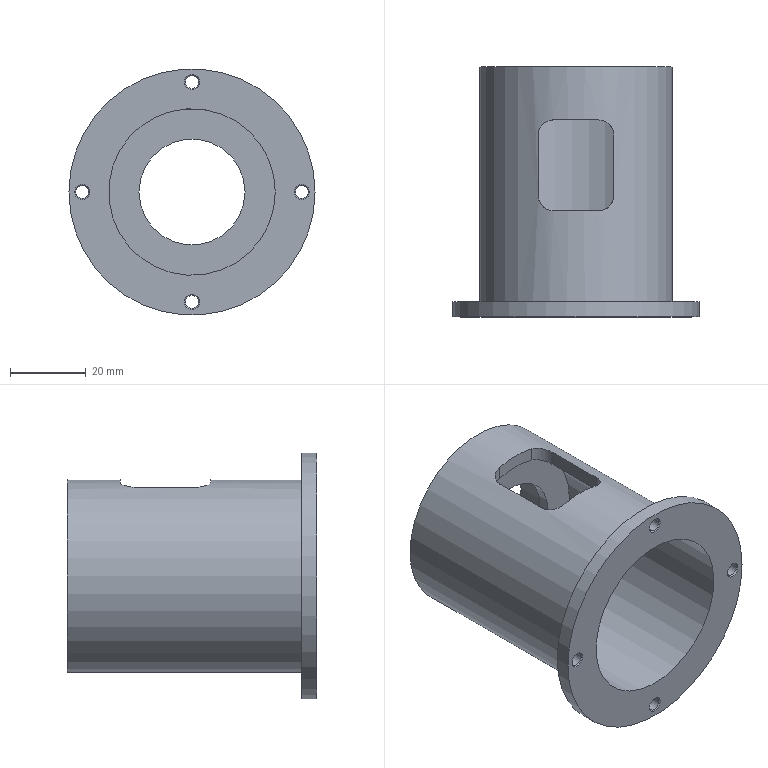Part | NX | features DATUM_CSYS 7, SKETCH 6, EXTRUDE 5, SIMPLE HOLE 4, BLEND 1, HOLE PACKAGE 1 | 1 solid | 30 faces | box 65 x 66 x 65 mm | volume 46902 mm3 | cylinder 13 | plane 9 | cone 8 | commonest cylinder face diameters 3.4 x4 8 x4 28 x1 32 x1 44 x1 51 x1
STEP:
#1=CARTESIAN_POINT('',(22.,54.,0.));
#2=VERTEX_POINT('',#1);
#3=CARTESIAN_POINT('',(0.,54.,0.));
#4=DIRECTION('',(0.,1.,0.));
#5=DIRECTION('',(1.,0.,0.));
#6=AXIS2_PLACEMENT_3D('',#3,#4,#5);
#7=CIRCLE('',#6,22.);
#8=EDGE_CURVE('',#2,#2,#7,.T.);
#9=ORIENTED_EDGE('',*,*,#8,.T.);
#10=EDGE_LOOP('',(#9));
#11=FACE_BOUND('',#10,.T.);
#12=CARTESIAN_POINT('',(22.,0.,0.));
#13=VERTEX_POINT('',#12);
#14=CARTESIAN_POINT('',(0.,0.,0.));
#15=DIRECTION('',(0.,-1.,0.));
#16=DIRECTION('',(1.,0.,0.));
#17=AXIS2_PLACEMENT_3D('',#14,#15,#16);
#18=CIRCLE('',#17,22.);
#19=EDGE_CURVE('',#13,#13,#18,.T.);
#20=ORIENTED_EDGE('',*,*,#19,.T.);
#21=EDGE_LOOP('',(#20));
#22=FACE_BOUND('',#21,.T.);
#23=CARTESIAN_POINT('',(-10.,32.,19.596));
#24=VERTEX_POINT('',#23);
#25=CARTESIAN_POINT('',(-10.,48.,19.596));
#26=VERTEX_POINT('',#25);
#27=CARTESIAN_POINT('',(-10.,4.,19.596));
#28=DIRECTION('',(0.,-1.,0.));
#29=VECTOR('',#28,1000.);
#30=LINE('',#27,#29);
#31=EDGE_CURVE('',#24,#26,#30,.F.);
#32=ORIENTED_EDGE('',*,*,#31,.F.);
#33=CARTESIAN_POINT('',(-6.,28.,21.166));
#34=VERTEX_POINT('',#33);
#35=CARTESIAN_POINT('',(-10.,32.,19.596));
#36=CARTESIAN_POINT('',(-10.,30.905,19.596));
#37=CARTESIAN_POINT('',(-9.065,28.825,20.099));
#38=CARTESIAN_POINT('',(-7.052,28.,20.868));
#39=CARTESIAN_POINT('',(-6.,28.,21.166));
#40=B_SPLINE_CURVE_WITH_KNOTS('',3,(#35,#36,#37,#38,#39),.UNSPECIFIED.,.F.,.F.,(4,1,4),(0.,0.003234,0.006469),.UNSPECIFIED.);
#41=EDGE_CURVE('',#24,#34,#40,.T.);
#42=ORIENTED_EDGE('',*,*,#41,.T.);
#43=CARTESIAN_POINT('',(6.,28.,21.166));
#44=VERTEX_POINT('',#43);
#45=CARTESIAN_POINT('',(0.,28.,0.));
#46=DIRECTION('',(0.,1.,0.));
#47=DIRECTION('',(0.,0.,1.));
#48=AXIS2_PLACEMENT_3D('',#45,#46,#47);
#49=CIRCLE('',#48,22.);
#50=EDGE_CURVE('',#44,#34,#49,.F.);
#51=ORIENTED_EDGE('',*,*,#50,.F.);
#52=CARTESIAN_POINT('',(10.,32.,19.596));
#53=VERTEX_POINT('',#52);
#54=CARTESIAN_POINT('',(6.,28.,21.166));
#55=CARTESIAN_POINT('',(7.053,28.,20.868));
#56=CARTESIAN_POINT('',(9.063,28.824,20.1));
#57=CARTESIAN_POINT('',(10.,30.904,19.596));
#58=CARTESIAN_POINT('',(10.,32.,19.596));
#59=B_SPLINE_CURVE_WITH_KNOTS('',3,(#54,#55,#56,#57,#58),.UNSPECIFIED.,.F.,.F.,(4,1,4),(0.,0.003235,0.006469),.UNSPECIFIED.);
#60=EDGE_CURVE('',#44,#53,#59,.T.);
#61=ORIENTED_EDGE('',*,*,#60,.T.);
#62=CARTESIAN_POINT('',(10.,48.,19.596));
#63=VERTEX_POINT('',#62);
#64=CARTESIAN_POINT('',(10.,4.,19.596));
#65=DIRECTION('',(0.,-1.,0.));
#66=VECTOR('',#65,1000.);
#67=LINE('',#64,#66);
#68=EDGE_CURVE('',#63,#53,#67,.T.);
#69=ORIENTED_EDGE('',*,*,#68,.F.);
#70=CARTESIAN_POINT('',(6.,52.,21.166));
#71=VERTEX_POINT('',#70);
#72=CARTESIAN_POINT('',(10.,48.,19.596));
#73=CARTESIAN_POINT('',(10.,49.095,19.596));
#74=CARTESIAN_POINT('',(9.065,51.175,20.099));
#75=CARTESIAN_POINT('',(7.052,52.,20.868));
#76=CARTESIAN_POINT('',(6.,52.,21.166));
#77=B_SPLINE_CURVE_WITH_KNOTS('',3,(#72,#73,#74,#75,#76),.UNSPECIFIED.,.F.,.F.,(4,1,4),(0.,0.003234,0.006469),.UNSPECIFIED.);
#78=EDGE_CURVE('',#63,#71,#77,.T.);
#79=ORIENTED_EDGE('',*,*,#78,.T.);
#80=CARTESIAN_POINT('',(-6.,52.,21.166));
#81=VERTEX_POINT('',#80);
#82=CARTESIAN_POINT('',(0.,52.,0.));
#83=DIRECTION('',(0.,-1.,0.));
#84=DIRECTION('',(0.,0.,-1.));
#85=AXIS2_PLACEMENT_3D('',#82,#83,#84);
#86=CIRCLE('',#85,22.);
#87=EDGE_CURVE('',#81,#71,#86,.F.);
#88=ORIENTED_EDGE('',*,*,#87,.F.);
#89=CARTESIAN_POINT('',(-6.,52.,21.166));
#90=CARTESIAN_POINT('',(-7.053,52.,20.868));
#91=CARTESIAN_POINT('',(-9.063,51.176,20.1));
#92=CARTESIAN_POINT('',(-10.,49.096,19.596));
#93=CARTESIAN_POINT('',(-10.,48.,19.596));
#94=B_SPLINE_CURVE_WITH_KNOTS('',3,(#89,#90,#91,#92,#93),.UNSPECIFIED.,.F.,.F.,(4,1,4),(0.,0.003235,0.006469),.UNSPECIFIED.);
#95=EDGE_CURVE('',#81,#26,#94,.T.);
#96=ORIENTED_EDGE('',*,*,#95,.T.);
#97=EDGE_LOOP('',(#32,#42,#51,#61,#69,#79,#88,#96));
#98=FACE_BOUND('',#97,.T.);
#99=CARTESIAN_POINT('',(0.,4.,0.));
#100=DIRECTION('',(0.,-1.,0.));
#101=DIRECTION('',(0.,0.,-1.));
#102=AXIS2_PLACEMENT_3D('',#99,#100,#101);
#103=CYLINDRICAL_SURFACE('',#102,22.);
#104=ADVANCED_FACE('',(#11,#22,#98),#103,.F.);
#105=CARTESIAN_POINT('',(25.5,66.,0.));
#106=VERTEX_POINT('',#105);
#107=CARTESIAN_POINT('',(0.,66.,0.));
#108=DIRECTION('',(0.,1.,0.));
#109=DIRECTION('',(1.,0.,0.));
#110=AXIS2_PLACEMENT_3D('',#107,#108,#109);
#111=CIRCLE('',#110,25.5);
#112=EDGE_CURVE('',#106,#106,#111,.T.);
#113=ORIENTED_EDGE('',*,*,#112,.F.);
#114=EDGE_LOOP('',(#113));
#115=FACE_BOUND('',#114,.T.);
#116=CARTESIAN_POINT('',(25.5,4.,0.));
#117=VERTEX_POINT('',#116);
#118=CARTESIAN_POINT('',(0.,4.,0.));
#119=DIRECTION('',(0.,1.,0.));
#120=DIRECTION('',(1.,0.,0.));
#121=AXIS2_PLACEMENT_3D('',#118,#119,#120);
#122=CIRCLE('',#121,25.5);
#123=EDGE_CURVE('',#117,#117,#122,.T.);
#124=ORIENTED_EDGE('',*,*,#123,.T.);
#125=EDGE_LOOP('',(#124));
#126=FACE_BOUND('',#125,.T.);
#127=CARTESIAN_POINT('',(-10.,48.,23.457));
#128=VERTEX_POINT('',#127);
#129=CARTESIAN_POINT('',(-10.,32.,23.457));
#130=VERTEX_POINT('',#129);
#131=CARTESIAN_POINT('',(-10.,54.,23.457));
#132=DIRECTION('',(0.,-1.,0.));
#133=VECTOR('',#132,1000.);
#134=LINE('',#131,#133);
#135=EDGE_CURVE('',#128,#130,#134,.T.);
#136=ORIENTED_EDGE('',*,*,#135,.F.);
#137=CARTESIAN_POINT('',(-6.,52.,24.784));
#138=VERTEX_POINT('',#137);
#139=CARTESIAN_POINT('',(-10.,48.,23.457));
#140=CARTESIAN_POINT('',(-10.,49.084,23.457));
#141=CARTESIAN_POINT('',(-9.082,51.163,23.871));
#142=CARTESIAN_POINT('',(-7.052,52.,24.529));
#143=CARTESIAN_POINT('',(-6.,52.,24.784));
#144=B_SPLINE_CURVE_WITH_KNOTS('',3,(#139,#140,#141,#142,#143),.UNSPECIFIED.,.F.,.F.,(4,1,4),(0.,0.003204,0.006407),.UNSPECIFIED.);
#145=EDGE_CURVE('',#128,#138,#144,.T.);
#146=ORIENTED_EDGE('',*,*,#145,.T.);
#147=CARTESIAN_POINT('',(6.,52.,24.784));
#148=VERTEX_POINT('',#147);
#149=CARTESIAN_POINT('',(0.,52.,0.));
#150=DIRECTION('',(0.,-1.,0.));
#151=DIRECTION('',(0.,0.,-1.));
#152=AXIS2_PLACEMENT_3D('',#149,#150,#151);
#153=CIRCLE('',#152,25.5);
#154=EDGE_CURVE('',#148,#138,#153,.T.);
#155=ORIENTED_EDGE('',*,*,#154,.F.);
#156=CARTESIAN_POINT('',(10.,48.,23.457));
#157=VERTEX_POINT('',#156);
#158=CARTESIAN_POINT('',(6.,52.,24.784));
#159=CARTESIAN_POINT('',(7.053,52.,24.529));
#160=CARTESIAN_POINT('',(9.079,51.165,23.871));
#161=CARTESIAN_POINT('',(10.,49.085,23.457));
#162=CARTESIAN_POINT('',(10.,48.,23.457));
#163=B_SPLINE_CURVE_WITH_KNOTS('',3,(#158,#159,#160,#161,#162),.UNSPECIFIED.,.F.,.F.,(4,1,4),(0.,0.003204,0.006407),.UNSPECIFIED.);
#164=EDGE_CURVE('',#148,#157,#163,.T.);
#165=ORIENTED_EDGE('',*,*,#164,.T.);
#166=CARTESIAN_POINT('',(10.,32.,23.457));
#167=VERTEX_POINT('',#166);
#168=CARTESIAN_POINT('',(10.,54.,23.457));
#169=DIRECTION('',(0.,-1.,0.));
#170=VECTOR('',#169,1000.);
#171=LINE('',#168,#170);
#172=EDGE_CURVE('',#167,#157,#171,.F.);
#173=ORIENTED_EDGE('',*,*,#172,.F.);
#174=CARTESIAN_POINT('',(6.,28.,24.784));
#175=VERTEX_POINT('',#174);
#176=CARTESIAN_POINT('',(10.,32.,23.457));
#177=CARTESIAN_POINT('',(10.,30.916,23.457));
#178=CARTESIAN_POINT('',(9.082,28.837,23.871));
#179=CARTESIAN_POINT('',(7.052,28.,24.529));
#180=CARTESIAN_POINT('',(6.,28.,24.784));
#181=B_SPLINE_CURVE_WITH_KNOTS('',3,(#176,#177,#178,#179,#180),.UNSPECIFIED.,.F.,.F.,(4,1,4),(0.,0.003204,0.006407),.UNSPECIFIED.);
#182=EDGE_CURVE('',#167,#175,#181,.T.);
#183=ORIENTED_EDGE('',*,*,#182,.T.);
#184=CARTESIAN_POINT('',(-6.,28.,24.784));
#185=VERTEX_POINT('',#184);
#186=CARTESIAN_POINT('',(0.,28.,0.));
#187=DIRECTION('',(0.,1.,0.));
#188=DIRECTION('',(0.,0.,1.));
#189=AXIS2_PLACEMENT_3D('',#186,#187,#188);
#190=CIRCLE('',#189,25.5);
#191=EDGE_CURVE('',#185,#175,#190,.T.);
#192=ORIENTED_EDGE('',*,*,#191,.F.);
#193=CARTESIAN_POINT('',(-6.,28.,24.784));
#194=CARTESIAN_POINT('',(-7.053,28.,24.529));
#195=CARTESIAN_POINT('',(-9.079,28.835,23.871));
#196=CARTESIAN_POINT('',(-10.,30.915,23.457));
#197=CARTESIAN_POINT('',(-10.,32.,23.457));
#198=B_SPLINE_CURVE_WITH_KNOTS('',3,(#193,#194,#195,#196,#197),.UNSPECIFIED.,.F.,.F.,(4,1,4),(0.,0.003204,0.006407),.UNSPECIFIED.);
#199=EDGE_CURVE('',#185,#130,#198,.T.);
#200=ORIENTED_EDGE('',*,*,#199,.T.);
#201=EDGE_LOOP('',(#136,#146,#155,#165,#173,#183,#192,#200));
#202=FACE_BOUND('',#201,.T.);
#203=CARTESIAN_POINT('',(0.,54.,0.));
#204=DIRECTION('',(0.,-1.,0.));
#205=DIRECTION('',(0.,0.,-1.));
#206=AXIS2_PLACEMENT_3D('',#203,#204,#205);
#207=CYLINDRICAL_SURFACE('',#206,25.5);
#208=ADVANCED_FACE('',(#115,#126,#202),#207,.T.);
#209=CARTESIAN_POINT('',(14.,57.,0.));
#210=VERTEX_POINT('',#209);
#211=CARTESIAN_POINT('',(0.,57.,0.));
#212=DIRECTION('',(0.,1.,0.));
#213=DIRECTION('',(1.,0.,0.));
#214=AXIS2_PLACEMENT_3D('',#211,#212,#213);
#215=CIRCLE('',#214,14.);
#216=EDGE_CURVE('',#210,#210,#215,.T.);
#217=ORIENTED_EDGE('',*,*,#216,.F.);
#218=EDGE_LOOP('',(#217));
#219=FACE_BOUND('',#218,.T.);
#220=CARTESIAN_POINT('',(16.,57.,0.));
#221=VERTEX_POINT('',#220);
#222=CARTESIAN_POINT('',(0.,57.,0.));
#223=DIRECTION('',(0.,1.,0.));
#224=DIRECTION('',(1.,0.,0.));
#225=AXIS2_PLACEMENT_3D('',#222,#223,#224);
#226=CIRCLE('',#225,16.);
#227=EDGE_CURVE('',#221,#221,#226,.T.);
#228=ORIENTED_EDGE('',*,*,#227,.T.);
#229=EDGE_LOOP('',(#228));
#230=FACE_BOUND('',#229,.T.);
#231=CARTESIAN_POINT('',(0.,57.,0.));
#232=DIRECTION('',(0.,1.,0.));
#233=DIRECTION('',(0.,0.,1.));
#234=AXIS2_PLACEMENT_3D('',#231,#232,#233);
#235=PLANE('',#234);
#236=ADVANCED_FACE('',(#219,#230),#235,.T.);
#237=CARTESIAN_POINT('',(29.,4.,-2.));
#238=VERTEX_POINT('',#237);
#239=CARTESIAN_POINT('',(29.,4.,0.));
#240=DIRECTION('',(0.,-1.,0.));
#241=DIRECTION('',(0.,0.,-1.));
#242=AXIS2_PLACEMENT_3D('',#239,#240,#241);
#243=CIRCLE('',#242,2.);
#244=EDGE_CURVE('',#238,#238,#243,.T.);
#245=ORIENTED_EDGE('',*,*,#244,.T.);
#246=EDGE_LOOP('',(#245));
#247=FACE_BOUND('',#246,.T.);
#248=CARTESIAN_POINT('',(0.,4.,27.));
#249=VERTEX_POINT('',#248);
#250=CARTESIAN_POINT('',(0.,4.,29.));
#251=DIRECTION('',(0.,-1.,0.));
#252=DIRECTION('',(0.,0.,-1.));
#253=AXIS2_PLACEMENT_3D('',#250,#251,#252);
#254=CIRCLE('',#253,2.);
#255=EDGE_CURVE('',#249,#249,#254,.T.);
#256=ORIENTED_EDGE('',*,*,#255,.T.);
#257=EDGE_LOOP('',(#256));
#258=FACE_BOUND('',#257,.T.);
#259=CARTESIAN_POINT('',(0.,4.,-31.));
#260=VERTEX_POINT('',#259);
#261=CARTESIAN_POINT('',(0.,4.,-29.));
#262=DIRECTION('',(0.,-1.,0.));
#263=DIRECTION('',(0.,0.,-1.));
#264=AXIS2_PLACEMENT_3D('',#261,#262,#263);
#265=CIRCLE('',#264,2.);
#266=EDGE_CURVE('',#260,#260,#265,.T.);
#267=ORIENTED_EDGE('',*,*,#266,.T.);
#268=EDGE_LOOP('',(#267));
#269=FACE_BOUND('',#268,.T.);
#270=CARTESIAN_POINT('',(-29.,4.,-2.));
#271=VERTEX_POINT('',#270);
#272=CARTESIAN_POINT('',(-29.,4.,0.));
#273=DIRECTION('',(0.,-1.,0.));
#274=DIRECTION('',(0.,0.,-1.));
#275=AXIS2_PLACEMENT_3D('',#272,#273,#274);
#276=CIRCLE('',#275,2.);
#277=EDGE_CURVE('',#271,#271,#276,.T.);
#278=ORIENTED_EDGE('',*,*,#277,.T.);
#279=EDGE_LOOP('',(#278));
#280=FACE_BOUND('',#279,.T.);
#281=CARTESIAN_POINT('',(32.5,4.,0.));
#282=VERTEX_POINT('',#281);
#283=CARTESIAN_POINT('',(0.,4.,0.));
#284=DIRECTION('',(0.,-1.,0.));
#285=DIRECTION('',(1.,0.,0.));
#286=AXIS2_PLACEMENT_3D('',#283,#284,#285);
#287=CIRCLE('',#286,32.5);
#288=EDGE_CURVE('',#282,#282,#287,.T.);
#289=ORIENTED_EDGE('',*,*,#288,.F.);
#290=EDGE_LOOP('',(#289));
#291=FACE_BOUND('',#290,.T.);
#292=ORIENTED_EDGE('',*,*,#123,.F.);
#293=EDGE_LOOP('',(#292));
#294=FACE_BOUND('',#293,.T.);
#295=CARTESIAN_POINT('',(0.,4.,0.));
#296=DIRECTION('',(0.,-1.,0.));
#297=DIRECTION('',(0.,0.,-1.));
#298=AXIS2_PLACEMENT_3D('',#295,#296,#297);
#299=PLANE('',#298);
#300=ADVANCED_FACE('',(#247,#258,#269,#280,#291,#294),#299,.F.);
#301=ORIENTED_EDGE('',*,*,#288,.T.);
#302=EDGE_LOOP('',(#301));
#303=FACE_BOUND('',#302,.T.);
#304=CARTESIAN_POINT('',(32.5,0.,0.));
#305=VERTEX_POINT('',#304);
#306=CARTESIAN_POINT('',(0.,0.,0.));
#307=DIRECTION('',(0.,-1.,0.));
#308=DIRECTION('',(1.,0.,0.));
#309=AXIS2_PLACEMENT_3D('',#306,#307,#308);
#310=CIRCLE('',#309,32.5);
#311=EDGE_CURVE('',#305,#305,#310,.T.);
#312=ORIENTED_EDGE('',*,*,#311,.F.);
#313=EDGE_LOOP('',(#312));
#314=FACE_BOUND('',#313,.T.);
#315=CARTESIAN_POINT('',(0.,4.,0.));
#316=DIRECTION('',(0.,-1.,0.));
#317=DIRECTION('',(0.,0.,-1.));
#318=AXIS2_PLACEMENT_3D('',#315,#316,#317);
#319=CYLINDRICAL_SURFACE('',#318,32.5);
#320=ADVANCED_FACE('',(#303,#314),#319,.T.);
#321=CARTESIAN_POINT('',(29.,0.,-2.));
#322=VERTEX_POINT('',#321);
#323=CARTESIAN_POINT('',(29.,0.,0.));
#324=DIRECTION('',(0.,-1.,0.));
#325=DIRECTION('',(0.,0.,-1.));
#326=AXIS2_PLACEMENT_3D('',#323,#324,#325);
#327=CIRCLE('',#326,2.);
#328=EDGE_CURVE('',#322,#322,#327,.F.);
#329=ORIENTED_EDGE('',*,*,#328,.T.);
#330=EDGE_LOOP('',(#329));
#331=FACE_BOUND('',#330,.T.);
#332=CARTESIAN_POINT('',(0.,0.,27.));
#333=VERTEX_POINT('',#332);
#334=CARTESIAN_POINT('',(0.,0.,29.));
#335=DIRECTION('',(0.,-1.,0.));
#336=DIRECTION('',(0.,0.,-1.));
#337=AXIS2_PLACEMENT_3D('',#334,#335,#336);
#338=CIRCLE('',#337,2.);
#339=EDGE_CURVE('',#333,#333,#338,.F.);
#340=ORIENTED_EDGE('',*,*,#339,.T.);
#341=EDGE_LOOP('',(#340));
#342=FACE_BOUND('',#341,.T.);
#343=CARTESIAN_POINT('',(0.,0.,-31.));
#344=VERTEX_POINT('',#343);
#345=CARTESIAN_POINT('',(0.,0.,-29.));
#346=DIRECTION('',(0.,-1.,0.));
#347=DIRECTION('',(0.,0.,-1.));
#348=AXIS2_PLACEMENT_3D('',#345,#346,#347);
#349=CIRCLE('',#348,2.);
#350=EDGE_CURVE('',#344,#344,#349,.F.);
#351=ORIENTED_EDGE('',*,*,#350,.T.);
#352=EDGE_LOOP('',(#351));
#353=FACE_BOUND('',#352,.T.);
#354=CARTESIAN_POINT('',(-29.,0.,-2.));
#355=VERTEX_POINT('',#354);
#356=CARTESIAN_POINT('',(-29.,0.,0.));
#357=DIRECTION('',(0.,-1.,0.));
#358=DIRECTION('',(0.,0.,-1.));
#359=AXIS2_PLACEMENT_3D('',#356,#357,#358);
#360=CIRCLE('',#359,2.);
#361=EDGE_CURVE('',#355,#355,#360,.F.);
#362=ORIENTED_EDGE('',*,*,#361,.T.);
#363=EDGE_LOOP('',(#362));
#364=FACE_BOUND('',#363,.T.);
#365=ORIENTED_EDGE('',*,*,#311,.T.);
#366=EDGE_LOOP('',(#365));
#367=FACE_BOUND('',#366,.T.);
#368=ORIENTED_EDGE('',*,*,#19,.F.);
#369=EDGE_LOOP('',(#368));
#370=FACE_BOUND('',#369,.T.);
#371=CARTESIAN_POINT('',(0.,0.,0.));
#372=DIRECTION('',(0.,-1.,0.));
#373=DIRECTION('',(0.,0.,-1.));
#374=AXIS2_PLACEMENT_3D('',#371,#372,#373);
#375=PLANE('',#374);
#376=ADVANCED_FACE('',(#331,#342,#353,#364,#367,#370),#375,.T.);
#377=ORIENTED_EDGE('',*,*,#216,.T.);
#378=EDGE_LOOP('',(#377));
#379=FACE_BOUND('',#378,.T.);
#380=CARTESIAN_POINT('',(14.,54.,0.));
#381=VERTEX_POINT('',#380);
#382=CARTESIAN_POINT('',(0.,54.,0.));
#383=DIRECTION('',(0.,1.,0.));
#384=DIRECTION('',(1.,0.,0.));
#385=AXIS2_PLACEMENT_3D('',#382,#383,#384);
#386=CIRCLE('',#385,14.);
#387=EDGE_CURVE('',#381,#381,#386,.T.);
#388=ORIENTED_EDGE('',*,*,#387,.F.);
#389=EDGE_LOOP('',(#388));
#390=FACE_BOUND('',#389,.T.);
#391=CARTESIAN_POINT('',(0.,57.,0.));
#392=DIRECTION('',(0.,-1.,0.));
#393=DIRECTION('',(0.,0.,-1.));
#394=AXIS2_PLACEMENT_3D('',#391,#392,#393);
#395=CYLINDRICAL_SURFACE('',#394,14.);
#396=ADVANCED_FACE('',(#379,#390),#395,.F.);
#397=ORIENTED_EDGE('',*,*,#8,.F.);
#398=EDGE_LOOP('',(#397));
#399=FACE_BOUND('',#398,.T.);
#400=ORIENTED_EDGE('',*,*,#387,.T.);
#401=EDGE_LOOP('',(#400));
#402=FACE_BOUND('',#401,.T.);
#403=CARTESIAN_POINT('',(0.,54.,0.));
#404=DIRECTION('',(0.,1.,0.));
#405=DIRECTION('',(0.,0.,1.));
#406=AXIS2_PLACEMENT_3D('',#403,#404,#405);
#407=PLANE('',#406);
#408=ADVANCED_FACE('',(#399,#402),#407,.F.);
#409=CARTESIAN_POINT('',(-29.,3.7,-1.7));
#410=VERTEX_POINT('',#409);
#411=CARTESIAN_POINT('',(-29.,3.7,0.));
#412=DIRECTION('',(0.,-1.,0.));
#413=DIRECTION('',(0.,0.,-1.));
#414=AXIS2_PLACEMENT_3D('',#411,#412,#413);
#415=CIRCLE('',#414,1.7);
#416=EDGE_CURVE('',#410,#410,#415,.F.);
#417=ORIENTED_EDGE('',*,*,#416,.T.);
#418=EDGE_LOOP('',(#417));
#419=FACE_BOUND('',#418,.T.);
#420=CARTESIAN_POINT('',(-29.,0.3,-1.7));
#421=VERTEX_POINT('',#420);
#422=CARTESIAN_POINT('',(-29.,0.3,0.));
#423=DIRECTION('',(0.,-1.,0.));
#424=DIRECTION('',(0.,0.,-1.));
#425=AXIS2_PLACEMENT_3D('',#422,#423,#424);
#426=CIRCLE('',#425,1.7);
#427=EDGE_CURVE('',#421,#421,#426,.T.);
#428=ORIENTED_EDGE('',*,*,#427,.T.);
#429=EDGE_LOOP('',(#428));
#430=FACE_BOUND('',#429,.T.);
#431=CARTESIAN_POINT('',(-29.,0.,0.));
#432=DIRECTION('',(0.,1.,0.));
#433=DIRECTION('',(0.,0.,1.));
#434=AXIS2_PLACEMENT_3D('',#431,#432,#433);
#435=CYLINDRICAL_SURFACE('',#434,1.7);
#436=ADVANCED_FACE('',(#419,#430),#435,.F.);
#437=ORIENTED_EDGE('',*,*,#427,.F.);
#438=EDGE_LOOP('',(#437));
#439=FACE_BOUND('',#438,.T.);
#440=ORIENTED_EDGE('',*,*,#361,.F.);
#441=EDGE_LOOP('',(#440));
#442=FACE_BOUND('',#441,.T.);
#443=CARTESIAN_POINT('',(-29.,0.,0.));
#444=DIRECTION('',(0.,-1.,0.));
#445=DIRECTION('',(0.,0.,-1.));
#446=AXIS2_PLACEMENT_3D('',#443,#444,#445);
#447=CONICAL_SURFACE('',#446,2.,0.7854);
#448=ADVANCED_FACE('',(#439,#442),#447,.F.);
#449=ORIENTED_EDGE('',*,*,#416,.F.);
#450=EDGE_LOOP('',(#449));
#451=FACE_BOUND('',#450,.T.);
#452=ORIENTED_EDGE('',*,*,#277,.F.);
#453=EDGE_LOOP('',(#452));
#454=FACE_BOUND('',#453,.T.);
#455=CARTESIAN_POINT('',(-29.,4.,0.));
#456=DIRECTION('',(0.,1.,0.));
#457=DIRECTION('',(0.,0.,1.));
#458=AXIS2_PLACEMENT_3D('',#455,#456,#457);
#459=CONICAL_SURFACE('',#458,2.,0.7854);
#460=ADVANCED_FACE('',(#451,#454),#459,.F.);
#461=CARTESIAN_POINT('',(0.,3.7,-30.7));
#462=VERTEX_POINT('',#461);
#463=CARTESIAN_POINT('',(0.,3.7,-29.));
#464=DIRECTION('',(0.,-1.,0.));
#465=DIRECTION('',(0.,0.,-1.));
#466=AXIS2_PLACEMENT_3D('',#463,#464,#465);
#467=CIRCLE('',#466,1.7);
#468=EDGE_CURVE('',#462,#462,#467,.F.);
#469=ORIENTED_EDGE('',*,*,#468,.T.);
#470=EDGE_LOOP('',(#469));
#471=FACE_BOUND('',#470,.T.);
#472=CARTESIAN_POINT('',(0.,0.3,-30.7));
#473=VERTEX_POINT('',#472);
#474=CARTESIAN_POINT('',(0.,0.3,-29.));
#475=DIRECTION('',(0.,-1.,0.));
#476=DIRECTION('',(0.,0.,-1.));
#477=AXIS2_PLACEMENT_3D('',#474,#475,#476);
#478=CIRCLE('',#477,1.7);
#479=EDGE_CURVE('',#473,#473,#478,.T.);
#480=ORIENTED_EDGE('',*,*,#479,.T.);
#481=EDGE_LOOP('',(#480));
#482=FACE_BOUND('',#481,.T.);
#483=CARTESIAN_POINT('',(0.,0.,-29.));
#484=DIRECTION('',(0.,1.,0.));
#485=DIRECTION('',(0.,0.,1.));
#486=AXIS2_PLACEMENT_3D('',#483,#484,#485);
#487=CYLINDRICAL_SURFACE('',#486,1.7);
#488=ADVANCED_FACE('',(#471,#482),#487,.F.);
#489=ORIENTED_EDGE('',*,*,#479,.F.);
#490=EDGE_LOOP('',(#489));
#491=FACE_BOUND('',#490,.T.);
#492=ORIENTED_EDGE('',*,*,#350,.F.);
#493=EDGE_LOOP('',(#492));
#494=FACE_BOUND('',#493,.T.);
#495=CARTESIAN_POINT('',(0.,0.,-29.));
#496=DIRECTION('',(0.,-1.,0.));
#497=DIRECTION('',(0.,0.,-1.));
#498=AXIS2_PLACEMENT_3D('',#495,#496,#497);
#499=CONICAL_SURFACE('',#498,2.,0.7854);
#500=ADVANCED_FACE('',(#491,#494),#499,.F.);
#501=ORIENTED_EDGE('',*,*,#468,.F.);
#502=EDGE_LOOP('',(#501));
#503=FACE_BOUND('',#502,.T.);
#504=ORIENTED_EDGE('',*,*,#266,.F.);
#505=EDGE_LOOP('',(#504));
#506=FACE_BOUND('',#505,.T.);
#507=CARTESIAN_POINT('',(0.,4.,-29.));
#508=DIRECTION('',(0.,1.,0.));
#509=DIRECTION('',(0.,0.,1.));
#510=AXIS2_PLACEMENT_3D('',#507,#508,#509);
#511=CONICAL_SURFACE('',#510,2.,0.7854);
#512=ADVANCED_FACE('',(#503,#506),#511,.F.);
#513=CARTESIAN_POINT('',(0.,3.7,27.3));
#514=VERTEX_POINT('',#513);
#515=CARTESIAN_POINT('',(0.,3.7,29.));
#516=DIRECTION('',(0.,-1.,0.));
#517=DIRECTION('',(0.,0.,-1.));
#518=AXIS2_PLACEMENT_3D('',#515,#516,#517);
#519=CIRCLE('',#518,1.7);
#520=EDGE_CURVE('',#514,#514,#519,.F.);
#521=ORIENTED_EDGE('',*,*,#520,.T.);
#522=EDGE_LOOP('',(#521));
#523=FACE_BOUND('',#522,.T.);
#524=CARTESIAN_POINT('',(0.,0.3,27.3));
#525=VERTEX_POINT('',#524);
#526=CARTESIAN_POINT('',(0.,0.3,29.));
#527=DIRECTION('',(0.,-1.,0.));
#528=DIRECTION('',(0.,0.,-1.));
#529=AXIS2_PLACEMENT_3D('',#526,#527,#528);
#530=CIRCLE('',#529,1.7);
#531=EDGE_CURVE('',#525,#525,#530,.T.);
#532=ORIENTED_EDGE('',*,*,#531,.T.);
#533=EDGE_LOOP('',(#532));
#534=FACE_BOUND('',#533,.T.);
#535=CARTESIAN_POINT('',(0.,0.,29.));
#536=DIRECTION('',(0.,1.,0.));
#537=DIRECTION('',(0.,0.,1.));
#538=AXIS2_PLACEMENT_3D('',#535,#536,#537);
#539=CYLINDRICAL_SURFACE('',#538,1.7);
#540=ADVANCED_FACE('',(#523,#534),#539,.F.);
#541=ORIENTED_EDGE('',*,*,#531,.F.);
#542=EDGE_LOOP('',(#541));
#543=FACE_BOUND('',#542,.T.);
#544=ORIENTED_EDGE('',*,*,#339,.F.);
#545=EDGE_LOOP('',(#544));
#546=FACE_BOUND('',#545,.T.);
#547=CARTESIAN_POINT('',(0.,0.,29.));
#548=DIRECTION('',(0.,-1.,0.));
#549=DIRECTION('',(0.,0.,-1.));
#550=AXIS2_PLACEMENT_3D('',#547,#548,#549);
#551=CONICAL_SURFACE('',#550,2.,0.7854);
#552=ADVANCED_FACE('',(#543,#546),#551,.F.);
#553=ORIENTED_EDGE('',*,*,#520,.F.);
#554=EDGE_LOOP('',(#553));
#555=FACE_BOUND('',#554,.T.);
#556=ORIENTED_EDGE('',*,*,#255,.F.);
#557=EDGE_LOOP('',(#556));
#558=FACE_BOUND('',#557,.T.);
#559=CARTESIAN_POINT('',(0.,4.,29.));
#560=DIRECTION('',(0.,1.,0.));
#561=DIRECTION('',(0.,0.,1.));
#562=AXIS2_PLACEMENT_3D('',#559,#560,#561);
#563=CONICAL_SURFACE('',#562,2.,0.7854);
#564=ADVANCED_FACE('',(#555,#558),#563,.F.);
#565=CARTESIAN_POINT('',(29.,3.7,-1.7));
#566=VERTEX_POINT('',#565);
#567=CARTESIAN_POINT('',(29.,3.7,0.));
#568=DIRECTION('',(0.,-1.,0.));
#569=DIRECTION('',(0.,0.,-1.));
#570=AXIS2_PLACEMENT_3D('',#567,#568,#569);
#571=CIRCLE('',#570,1.7);
#572=EDGE_CURVE('',#566,#566,#571,.F.);
#573=ORIENTED_EDGE('',*,*,#572,.T.);
#574=EDGE_LOOP('',(#573));
#575=FACE_BOUND('',#574,.T.);
#576=CARTESIAN_POINT('',(29.,0.3,-1.7));
#577=VERTEX_POINT('',#576);
#578=CARTESIAN_POINT('',(29.,0.3,0.));
#579=DIRECTION('',(0.,-1.,0.));
#580=DIRECTION('',(0.,0.,-1.));
#581=AXIS2_PLACEMENT_3D('',#578,#579,#580);
#582=CIRCLE('',#581,1.7);
#583=EDGE_CURVE('',#577,#577,#582,.T.);
#584=ORIENTED_EDGE('',*,*,#583,.T.);
#585=EDGE_LOOP('',(#584));
#586=FACE_BOUND('',#585,.T.);
#587=CARTESIAN_POINT('',(29.,0.,0.));
#588=DIRECTION('',(0.,1.,0.));
#589=DIRECTION('',(0.,0.,1.));
#590=AXIS2_PLACEMENT_3D('',#587,#588,#589);
#591=CYLINDRICAL_SURFACE('',#590,1.7);
#592=ADVANCED_FACE('',(#575,#586),#591,.F.);
#593=ORIENTED_EDGE('',*,*,#583,.F.);
#594=EDGE_LOOP('',(#593));
#595=FACE_BOUND('',#594,.T.);
#596=ORIENTED_EDGE('',*,*,#328,.F.);
#597=EDGE_LOOP('',(#596));
#598=FACE_BOUND('',#597,.T.);
#599=CARTESIAN_POINT('',(29.,0.,0.));
#600=DIRECTION('',(0.,-1.,0.));
#601=DIRECTION('',(0.,0.,-1.));
#602=AXIS2_PLACEMENT_3D('',#599,#600,#601);
#603=CONICAL_SURFACE('',#602,2.,0.7854);
#604=ADVANCED_FACE('',(#595,#598),#603,.F.);
#605=ORIENTED_EDGE('',*,*,#572,.F.);
#606=EDGE_LOOP('',(#605));
#607=FACE_BOUND('',#606,.T.);
#608=ORIENTED_EDGE('',*,*,#244,.F.);
#609=EDGE_LOOP('',(#608));
#610=FACE_BOUND('',#609,.T.);
#611=CARTESIAN_POINT('',(29.,4.,0.));
#612=DIRECTION('',(0.,1.,0.));
#613=DIRECTION('',(0.,0.,1.));
#614=AXIS2_PLACEMENT_3D('',#611,#612,#613);
#615=CONICAL_SURFACE('',#614,2.,0.7854);
#616=ADVANCED_FACE('',(#607,#610),#615,.F.);
#617=CARTESIAN_POINT('',(16.,66.,0.));
#618=VERTEX_POINT('',#617);
#619=CARTESIAN_POINT('',(0.,66.,0.));
#620=DIRECTION('',(0.,1.,0.));
#621=DIRECTION('',(1.,0.,0.));
#622=AXIS2_PLACEMENT_3D('',#619,#620,#621);
#623=CIRCLE('',#622,16.);
#624=EDGE_CURVE('',#618,#618,#623,.T.);
#625=ORIENTED_EDGE('',*,*,#624,.T.);
#626=EDGE_LOOP('',(#625));
#627=FACE_BOUND('',#626,.T.);
#628=ORIENTED_EDGE('',*,*,#227,.F.);
#629=EDGE_LOOP('',(#628));
#630=FACE_BOUND('',#629,.T.);
#631=CARTESIAN_POINT('',(0.,66.,0.));
#632=DIRECTION('',(0.,-1.,0.));
#633=DIRECTION('',(0.,0.,-1.));
#634=AXIS2_PLACEMENT_3D('',#631,#632,#633);
#635=CYLINDRICAL_SURFACE('',#634,16.);
#636=ADVANCED_FACE('',(#627,#630),#635,.F.);
#637=ORIENTED_EDGE('',*,*,#112,.T.);
#638=EDGE_LOOP('',(#637));
#639=FACE_BOUND('',#638,.T.);
#640=ORIENTED_EDGE('',*,*,#624,.F.);
#641=EDGE_LOOP('',(#640));
#642=FACE_BOUND('',#641,.T.);
#643=CARTESIAN_POINT('',(0.,66.,0.));
#644=DIRECTION('',(0.,1.,0.));
#645=DIRECTION('',(0.,0.,1.));
#646=AXIS2_PLACEMENT_3D('',#643,#644,#645);
#647=PLANE('',#646);
#648=ADVANCED_FACE('',(#639,#642),#647,.T.);
#649=ORIENTED_EDGE('',*,*,#135,.T.);
#650=CARTESIAN_POINT('',(-10.,32.,19.596));
#651=DIRECTION('',(0.,0.,1.));
#652=VECTOR('',#651,1000.);
#653=LINE('',#650,#652);
#654=EDGE_CURVE('',#130,#24,#653,.F.);
#655=ORIENTED_EDGE('',*,*,#654,.T.);
#656=ORIENTED_EDGE('',*,*,#31,.T.);
#657=CARTESIAN_POINT('',(-10.,48.,23.457));
#658=DIRECTION('',(0.,0.,1.));
#659=VECTOR('',#658,1000.);
#660=LINE('',#657,#659);
#661=EDGE_CURVE('',#26,#128,#660,.T.);
#662=ORIENTED_EDGE('',*,*,#661,.T.);
#663=EDGE_LOOP('',(#649,#655,#656,#662));
#664=FACE_BOUND('',#663,.T.);
#665=CARTESIAN_POINT('',(-10.,52.,50.));
#666=DIRECTION('',(1.,0.,0.));
#667=DIRECTION('',(0.,1.,0.));
#668=AXIS2_PLACEMENT_3D('',#665,#666,#667);
#669=PLANE('',#668);
#670=ADVANCED_FACE('',(#664),#669,.T.);
#671=ORIENTED_EDGE('',*,*,#191,.T.);
#672=CARTESIAN_POINT('',(6.,28.,19.596));
#673=DIRECTION('',(0.,0.,1.));
#674=VECTOR('',#673,1000.);
#675=LINE('',#672,#674);
#676=EDGE_CURVE('',#175,#44,#675,.F.);
#677=ORIENTED_EDGE('',*,*,#676,.T.);
#678=ORIENTED_EDGE('',*,*,#50,.T.);
#679=CARTESIAN_POINT('',(-6.,28.,23.457));
#680=DIRECTION('',(0.,0.,1.));
#681=VECTOR('',#680,1000.);
#682=LINE('',#679,#681);
#683=EDGE_CURVE('',#34,#185,#682,.T.);
#684=ORIENTED_EDGE('',*,*,#683,.T.);
#685=EDGE_LOOP('',(#671,#677,#678,#684));
#686=FACE_BOUND('',#685,.T.);
#687=CARTESIAN_POINT('',(-10.,28.,50.));
#688=DIRECTION('',(0.,1.,0.));
#689=DIRECTION('',(0.,0.,1.));
#690=AXIS2_PLACEMENT_3D('',#687,#688,#689);
#691=PLANE('',#690);
#692=ADVANCED_FACE('',(#686),#691,.T.);
#693=ORIENTED_EDGE('',*,*,#172,.T.);
#694=CARTESIAN_POINT('',(10.,48.,19.596));
#695=DIRECTION('',(0.,0.,1.));
#696=VECTOR('',#695,1000.);
#697=LINE('',#694,#696);
#698=EDGE_CURVE('',#157,#63,#697,.F.);
#699=ORIENTED_EDGE('',*,*,#698,.T.);
#700=ORIENTED_EDGE('',*,*,#68,.T.);
#701=CARTESIAN_POINT('',(10.,32.,23.457));
#702=DIRECTION('',(0.,0.,1.));
#703=VECTOR('',#702,1000.);
#704=LINE('',#701,#703);
#705=EDGE_CURVE('',#53,#167,#704,.T.);
#706=ORIENTED_EDGE('',*,*,#705,.T.);
#707=EDGE_LOOP('',(#693,#699,#700,#706));
#708=FACE_BOUND('',#707,.T.);
#709=CARTESIAN_POINT('',(10.,28.,50.));
#710=DIRECTION('',(-1.,0.,0.));
#711=DIRECTION('',(0.,-1.,0.));
#712=AXIS2_PLACEMENT_3D('',#709,#710,#711);
#713=PLANE('',#712);
#714=ADVANCED_FACE('',(#708),#713,.T.);
#715=ORIENTED_EDGE('',*,*,#87,.T.);
#716=CARTESIAN_POINT('',(6.,52.,23.457));
#717=DIRECTION('',(0.,0.,1.));
#718=VECTOR('',#717,1000.);
#719=LINE('',#716,#718);
#720=EDGE_CURVE('',#71,#148,#719,.T.);
#721=ORIENTED_EDGE('',*,*,#720,.T.);
#722=ORIENTED_EDGE('',*,*,#154,.T.);
#723=CARTESIAN_POINT('',(-6.,52.,19.596));
#724=DIRECTION('',(0.,0.,1.));
#725=VECTOR('',#724,1000.);
#726=LINE('',#723,#725);
#727=EDGE_CURVE('',#138,#81,#726,.F.);
#728=ORIENTED_EDGE('',*,*,#727,.T.);
#729=EDGE_LOOP('',(#715,#721,#722,#728));
#730=FACE_BOUND('',#729,.T.);
#731=CARTESIAN_POINT('',(10.,52.,50.));
#732=DIRECTION('',(0.,-1.,0.));
#733=DIRECTION('',(0.,0.,-1.));
#734=AXIS2_PLACEMENT_3D('',#731,#732,#733);
#735=PLANE('',#734);
#736=ADVANCED_FACE('',(#730),#735,.T.);
#737=ORIENTED_EDGE('',*,*,#78,.F.);
#738=ORIENTED_EDGE('',*,*,#698,.F.);
#739=ORIENTED_EDGE('',*,*,#164,.F.);
#740=ORIENTED_EDGE('',*,*,#720,.F.);
#741=EDGE_LOOP('',(#737,#738,#739,#740));
#742=FACE_BOUND('',#741,.T.);
#743=CARTESIAN_POINT('',(6.,48.,50.));
#744=DIRECTION('',(0.,0.,-1.));
#745=DIRECTION('',(-1.,0.,0.));
#746=AXIS2_PLACEMENT_3D('',#743,#744,#745);
#747=CYLINDRICAL_SURFACE('',#746,4.);
#748=ADVANCED_FACE('',(#742),#747,.F.);
#749=ORIENTED_EDGE('',*,*,#60,.F.);
#750=ORIENTED_EDGE('',*,*,#676,.F.);
#751=ORIENTED_EDGE('',*,*,#182,.F.);
#752=ORIENTED_EDGE('',*,*,#705,.F.);
#753=EDGE_LOOP('',(#749,#750,#751,#752));
#754=FACE_BOUND('',#753,.T.);
#755=CARTESIAN_POINT('',(6.,32.,50.));
#756=DIRECTION('',(0.,0.,-1.));
#757=DIRECTION('',(-1.,0.,0.));
#758=AXIS2_PLACEMENT_3D('',#755,#756,#757);
#759=CYLINDRICAL_SURFACE('',#758,4.);
#760=ADVANCED_FACE('',(#754),#759,.F.);
#761=ORIENTED_EDGE('',*,*,#41,.F.);
#762=ORIENTED_EDGE('',*,*,#654,.F.);
#763=ORIENTED_EDGE('',*,*,#199,.F.);
#764=ORIENTED_EDGE('',*,*,#683,.F.);
#765=EDGE_LOOP('',(#761,#762,#763,#764));
#766=FACE_BOUND('',#765,.T.);
#767=CARTESIAN_POINT('',(-6.,32.,50.));
#768=DIRECTION('',(0.,0.,-1.));
#769=DIRECTION('',(-1.,0.,0.));
#770=AXIS2_PLACEMENT_3D('',#767,#768,#769);
#771=CYLINDRICAL_SURFACE('',#770,4.);
#772=ADVANCED_FACE('',(#766),#771,.F.);
#773=ORIENTED_EDGE('',*,*,#95,.F.);
#774=ORIENTED_EDGE('',*,*,#727,.F.);
#775=ORIENTED_EDGE('',*,*,#145,.F.);
#776=ORIENTED_EDGE('',*,*,#661,.F.);
#777=EDGE_LOOP('',(#773,#774,#775,#776));
#778=FACE_BOUND('',#777,.T.);
#779=CARTESIAN_POINT('',(-6.,48.,50.));
#780=DIRECTION('',(0.,0.,-1.));
#781=DIRECTION('',(-1.,0.,0.));
#782=AXIS2_PLACEMENT_3D('',#779,#780,#781);
#783=CYLINDRICAL_SURFACE('',#782,4.);
#784=ADVANCED_FACE('',(#778),#783,.F.);
#785=CLOSED_SHELL('',(#104,#208,#236,#300,#320,#376,#396,#408,#436,#448,#460,#488,#500,#512,#540,#552,#564,#592,#604,#616,#636,#648,#670,#692,#714,#736,#748,#760,#772,#784));
#786=MANIFOLD_SOLID_BREP('',#785);
#787=(LENGTH_UNIT()NAMED_UNIT(*)SI_UNIT(.MILLI.,.METRE.));
#788=UNCERTAINTY_MEASURE_WITH_UNIT(LENGTH_MEASURE(0.0508),#787,'','');
#789=(NAMED_UNIT(*)PLANE_ANGLE_UNIT()SI_UNIT($,.RADIAN.));
#790=(NAMED_UNIT(*)SI_UNIT($,.STERADIAN.)SOLID_ANGLE_UNIT());
#791=(GEOMETRIC_REPRESENTATION_CONTEXT(3)GLOBAL_UNCERTAINTY_ASSIGNED_CONTEXT((#788))GLOBAL_UNIT_ASSIGNED_CONTEXT((#787,#789,#790))REPRESENTATION_CONTEXT('',''));
#792=ADVANCED_BREP_SHAPE_REPRESENTATION('',(#786),#791);